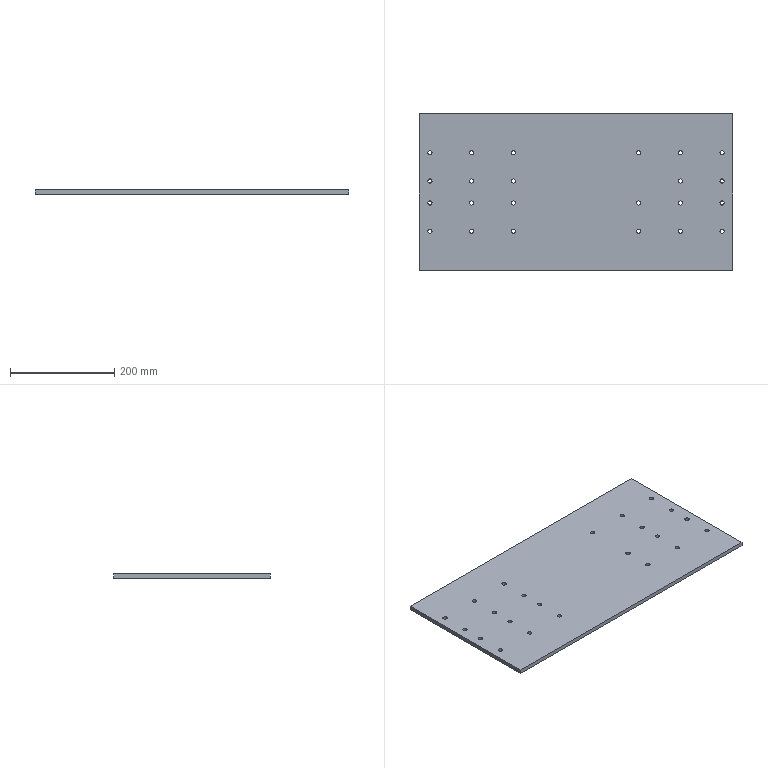Part | STEP file | 01-Top plate | 1 solid | 52 faces | box 600 x 300 x 8 mm | volume 1430751 mm3 | cylinder 46 | plane 6 | commonest cylinder face diameters 8 x46